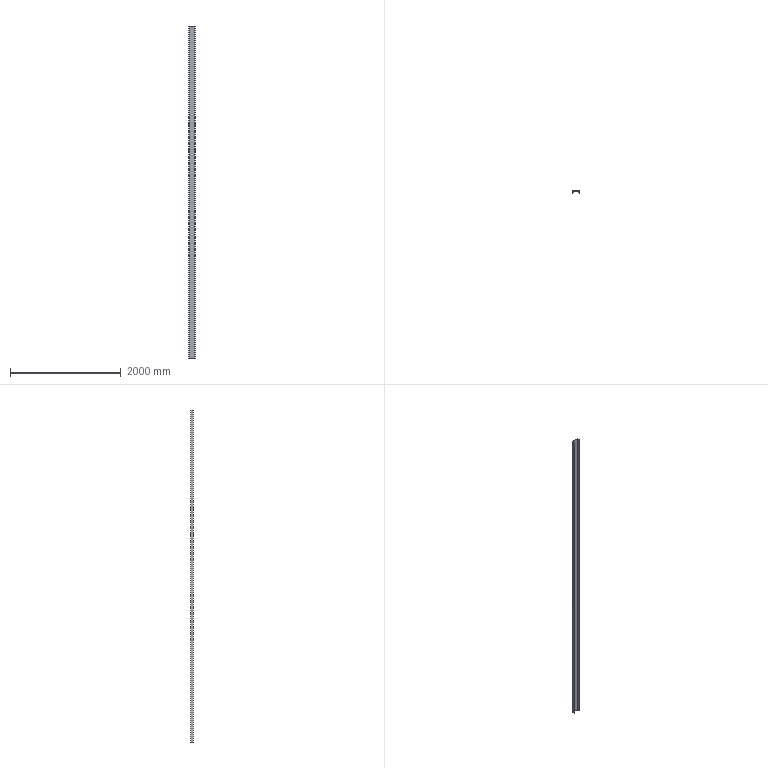Part | SolidWorks | features Extrusion 1 | 1 solid | 14 faces | box 120 x 50 x 6000 mm | volume 8487812 mm3 | plane 10 | cylinder 4 | commonest cylinder face diameters 4 x2 10 x2
STEP:
#1=CARTESIAN_POINT('',(0.,0.,0.));
#2=VERTEX_POINT('',#1);
#3=CARTESIAN_POINT('',(2.549,0.,0.));
#4=VERTEX_POINT('',#3);
#5=CARTESIAN_POINT('',(0.,0.,0.));
#6=DIRECTION('',(1.,0.,0.));
#7=VECTOR('',#6,1000.);
#8=LINE('',#5,#7);
#9=EDGE_CURVE('',#2,#4,#8,.T.);
#10=ORIENTED_EDGE('',*,*,#9,.T.);
#11=CARTESIAN_POINT('',(2.549,0.,6000.));
#12=VERTEX_POINT('',#11);
#13=CARTESIAN_POINT('',(2.549,0.,6000.));
#14=DIRECTION('',(0.,0.,-1.));
#15=VECTOR('',#14,1000.);
#16=LINE('',#13,#15);
#17=EDGE_CURVE('',#12,#4,#16,.T.);
#18=ORIENTED_EDGE('',*,*,#17,.F.);
#19=CARTESIAN_POINT('',(0.,0.,6000.));
#20=VERTEX_POINT('',#19);
#21=CARTESIAN_POINT('',(0.,0.,6000.));
#22=DIRECTION('',(1.,0.,0.));
#23=VECTOR('',#22,1000.);
#24=LINE('',#21,#23);
#25=EDGE_CURVE('',#20,#12,#24,.T.);
#26=ORIENTED_EDGE('',*,*,#25,.F.);
#27=CARTESIAN_POINT('',(0.,0.,6000.));
#28=DIRECTION('',(0.,0.,-1.));
#29=VECTOR('',#28,1000.);
#30=LINE('',#27,#29);
#31=EDGE_CURVE('',#20,#2,#30,.T.);
#32=ORIENTED_EDGE('',*,*,#31,.T.);
#33=EDGE_LOOP('',(#10,#18,#26,#32));
#34=FACE_OUTER_BOUND('',#33,.T.);
#35=CARTESIAN_POINT('',(0.,0.,6000.));
#36=DIRECTION('',(0.,1.,0.));
#37=DIRECTION('',(0.,0.,1.));
#38=AXIS2_PLACEMENT_3D('',#35,#36,#37);
#39=PLANE('',#38);
#40=ADVANCED_FACE('',(#34),#39,.F.);
#41=CARTESIAN_POINT('',(4.536,1.773,0.));
#42=VERTEX_POINT('',#41);
#43=CARTESIAN_POINT('',(2.549,2.,0.));
#44=DIRECTION('',(0.,0.,1.));
#45=DIRECTION('',(-1.,0.,0.));
#46=AXIS2_PLACEMENT_3D('',#43,#44,#45);
#47=CIRCLE('',#46,2.);
#48=EDGE_CURVE('',#4,#42,#47,.T.);
#49=ORIENTED_EDGE('',*,*,#48,.T.);
#50=CARTESIAN_POINT('',(4.536,1.773,6000.));
#51=VERTEX_POINT('',#50);
#52=CARTESIAN_POINT('',(4.536,1.773,6000.));
#53=DIRECTION('',(0.,0.,-1.));
#54=VECTOR('',#53,1000.);
#55=LINE('',#52,#54);
#56=EDGE_CURVE('',#51,#42,#55,.T.);
#57=ORIENTED_EDGE('',*,*,#56,.F.);
#58=CARTESIAN_POINT('',(2.549,2.,6000.));
#59=DIRECTION('',(0.,0.,1.));
#60=DIRECTION('',(-1.,0.,0.));
#61=AXIS2_PLACEMENT_3D('',#58,#59,#60);
#62=CIRCLE('',#61,2.);
#63=EDGE_CURVE('',#12,#51,#62,.T.);
#64=ORIENTED_EDGE('',*,*,#63,.F.);
#65=ORIENTED_EDGE('',*,*,#17,.T.);
#66=EDGE_LOOP('',(#49,#57,#64,#65));
#67=FACE_OUTER_BOUND('',#66,.T.);
#68=CARTESIAN_POINT('',(2.549,2.,6000.));
#69=DIRECTION('',(0.,0.,-1.));
#70=DIRECTION('',(-1.,0.,0.));
#71=AXIS2_PLACEMENT_3D('',#68,#69,#70);
#72=CYLINDRICAL_SURFACE('',#71,2.);
#73=ADVANCED_FACE('',(#67),#72,.T.);
#74=CARTESIAN_POINT('',(8.753,38.724,0.));
#75=VERTEX_POINT('',#74);
#76=CARTESIAN_POINT('',(4.536,1.773,0.));
#77=DIRECTION('',(0.1134,0.9936,0.));
#78=VECTOR('',#77,1000.);
#79=LINE('',#76,#78);
#80=EDGE_CURVE('',#42,#75,#79,.T.);
#81=ORIENTED_EDGE('',*,*,#80,.T.);
#82=CARTESIAN_POINT('',(8.753,38.724,6000.));
#83=VERTEX_POINT('',#82);
#84=CARTESIAN_POINT('',(8.753,38.724,6000.));
#85=DIRECTION('',(0.,0.,-1.));
#86=VECTOR('',#85,1000.);
#87=LINE('',#84,#86);
#88=EDGE_CURVE('',#83,#75,#87,.T.);
#89=ORIENTED_EDGE('',*,*,#88,.F.);
#90=CARTESIAN_POINT('',(4.536,1.773,6000.));
#91=DIRECTION('',(0.1134,0.9936,0.));
#92=VECTOR('',#91,1000.);
#93=LINE('',#90,#92);
#94=EDGE_CURVE('',#51,#83,#93,.T.);
#95=ORIENTED_EDGE('',*,*,#94,.F.);
#96=ORIENTED_EDGE('',*,*,#56,.T.);
#97=EDGE_LOOP('',(#81,#89,#95,#96));
#98=FACE_OUTER_BOUND('',#97,.T.);
#99=CARTESIAN_POINT('',(4.536,1.773,6000.));
#100=DIRECTION('',(-0.9936,0.1134,0.));
#101=DIRECTION('',(-0.1134,-0.9936,0.));
#102=AXIS2_PLACEMENT_3D('',#99,#100,#101);
#103=PLANE('',#102);
#104=ADVANCED_FACE('',(#98),#103,.F.);
#105=CARTESIAN_POINT('',(13.72,43.157,0.));
#106=VERTEX_POINT('',#105);
#107=CARTESIAN_POINT('',(13.72,38.157,0.));
#108=DIRECTION('',(0.,0.,-1.));
#109=DIRECTION('',(-1.,0.,0.));
#110=AXIS2_PLACEMENT_3D('',#107,#108,#109);
#111=CIRCLE('',#110,5.);
#112=EDGE_CURVE('',#75,#106,#111,.T.);
#113=ORIENTED_EDGE('',*,*,#112,.T.);
#114=CARTESIAN_POINT('',(13.72,43.157,6000.));
#115=VERTEX_POINT('',#114);
#116=CARTESIAN_POINT('',(13.72,43.157,6000.));
#117=DIRECTION('',(0.,0.,-1.));
#118=VECTOR('',#117,1000.);
#119=LINE('',#116,#118);
#120=EDGE_CURVE('',#115,#106,#119,.T.);
#121=ORIENTED_EDGE('',*,*,#120,.F.);
#122=CARTESIAN_POINT('',(13.72,38.157,6000.));
#123=DIRECTION('',(0.,0.,-1.));
#124=DIRECTION('',(-1.,0.,0.));
#125=AXIS2_PLACEMENT_3D('',#122,#123,#124);
#126=CIRCLE('',#125,5.);
#127=EDGE_CURVE('',#83,#115,#126,.T.);
#128=ORIENTED_EDGE('',*,*,#127,.F.);
#129=ORIENTED_EDGE('',*,*,#88,.T.);
#130=EDGE_LOOP('',(#113,#121,#128,#129));
#131=FACE_OUTER_BOUND('',#130,.T.);
#132=CARTESIAN_POINT('',(13.72,38.157,6000.));
#133=DIRECTION('',(0.,0.,-1.));
#134=DIRECTION('',(-1.,0.,0.));
#135=AXIS2_PLACEMENT_3D('',#132,#133,#134);
#136=CYLINDRICAL_SURFACE('',#135,5.);
#137=ADVANCED_FACE('',(#131),#136,.F.);
#138=CARTESIAN_POINT('',(106.28,43.157,0.));
#139=VERTEX_POINT('',#138);
#140=CARTESIAN_POINT('',(13.72,43.157,0.));
#141=DIRECTION('',(1.,0.,0.));
#142=VECTOR('',#141,1000.);
#143=LINE('',#140,#142);
#144=EDGE_CURVE('',#106,#139,#143,.T.);
#145=ORIENTED_EDGE('',*,*,#144,.T.);
#146=CARTESIAN_POINT('',(106.28,43.157,6000.));
#147=VERTEX_POINT('',#146);
#148=CARTESIAN_POINT('',(106.28,43.157,6000.));
#149=DIRECTION('',(0.,0.,-1.));
#150=VECTOR('',#149,1000.);
#151=LINE('',#148,#150);
#152=EDGE_CURVE('',#147,#139,#151,.T.);
#153=ORIENTED_EDGE('',*,*,#152,.F.);
#154=CARTESIAN_POINT('',(13.72,43.157,6000.));
#155=DIRECTION('',(1.,0.,0.));
#156=VECTOR('',#155,1000.);
#157=LINE('',#154,#156);
#158=EDGE_CURVE('',#115,#147,#157,.T.);
#159=ORIENTED_EDGE('',*,*,#158,.F.);
#160=ORIENTED_EDGE('',*,*,#120,.T.);
#161=EDGE_LOOP('',(#145,#153,#159,#160));
#162=FACE_OUTER_BOUND('',#161,.T.);
#163=CARTESIAN_POINT('',(13.72,43.157,6000.));
#164=DIRECTION('',(0.,1.,0.));
#165=DIRECTION('',(0.,0.,1.));
#166=AXIS2_PLACEMENT_3D('',#163,#164,#165);
#167=PLANE('',#166);
#168=ADVANCED_FACE('',(#162),#167,.F.);
#169=CARTESIAN_POINT('',(111.247,38.724,0.));
#170=VERTEX_POINT('',#169);
#171=CARTESIAN_POINT('',(106.28,38.157,0.));
#172=DIRECTION('',(0.,0.,-1.));
#173=DIRECTION('',(1.,0.,0.));
#174=AXIS2_PLACEMENT_3D('',#171,#172,#173);
#175=CIRCLE('',#174,5.);
#176=EDGE_CURVE('',#139,#170,#175,.T.);
#177=ORIENTED_EDGE('',*,*,#176,.T.);
#178=CARTESIAN_POINT('',(111.247,38.724,6000.));
#179=VERTEX_POINT('',#178);
#180=CARTESIAN_POINT('',(111.247,38.724,6000.));
#181=DIRECTION('',(0.,0.,-1.));
#182=VECTOR('',#181,1000.);
#183=LINE('',#180,#182);
#184=EDGE_CURVE('',#179,#170,#183,.T.);
#185=ORIENTED_EDGE('',*,*,#184,.F.);
#186=CARTESIAN_POINT('',(106.28,38.157,6000.));
#187=DIRECTION('',(0.,0.,-1.));
#188=DIRECTION('',(1.,0.,0.));
#189=AXIS2_PLACEMENT_3D('',#186,#187,#188);
#190=CIRCLE('',#189,5.);
#191=EDGE_CURVE('',#147,#179,#190,.T.);
#192=ORIENTED_EDGE('',*,*,#191,.F.);
#193=ORIENTED_EDGE('',*,*,#152,.T.);
#194=EDGE_LOOP('',(#177,#185,#192,#193));
#195=FACE_OUTER_BOUND('',#194,.T.);
#196=CARTESIAN_POINT('',(106.28,38.157,6000.));
#197=DIRECTION('',(0.,0.,-1.));
#198=DIRECTION('',(-1.,0.,0.));
#199=AXIS2_PLACEMENT_3D('',#196,#197,#198);
#200=CYLINDRICAL_SURFACE('',#199,5.);
#201=ADVANCED_FACE('',(#195),#200,.F.);
#202=CARTESIAN_POINT('',(115.464,1.773,0.));
#203=VERTEX_POINT('',#202);
#204=CARTESIAN_POINT('',(115.464,1.773,0.));
#205=DIRECTION('',(0.1134,-0.9936,0.));
#206=VECTOR('',#205,1000.);
#207=LINE('',#204,#206);
#208=EDGE_CURVE('',#170,#203,#207,.T.);
#209=ORIENTED_EDGE('',*,*,#208,.T.);
#210=CARTESIAN_POINT('',(115.464,1.773,6000.));
#211=VERTEX_POINT('',#210);
#212=CARTESIAN_POINT('',(115.464,1.773,6000.));
#213=DIRECTION('',(0.,0.,-1.));
#214=VECTOR('',#213,1000.);
#215=LINE('',#212,#214);
#216=EDGE_CURVE('',#211,#203,#215,.T.);
#217=ORIENTED_EDGE('',*,*,#216,.F.);
#218=CARTESIAN_POINT('',(115.464,1.773,6000.));
#219=DIRECTION('',(0.1134,-0.9936,0.));
#220=VECTOR('',#219,1000.);
#221=LINE('',#218,#220);
#222=EDGE_CURVE('',#179,#211,#221,.T.);
#223=ORIENTED_EDGE('',*,*,#222,.F.);
#224=ORIENTED_EDGE('',*,*,#184,.T.);
#225=EDGE_LOOP('',(#209,#217,#223,#224));
#226=FACE_OUTER_BOUND('',#225,.T.);
#227=CARTESIAN_POINT('',(115.464,1.773,6000.));
#228=DIRECTION('',(0.9936,0.1134,0.));
#229=DIRECTION('',(-0.1134,0.9936,0.));
#230=AXIS2_PLACEMENT_3D('',#227,#228,#229);
#231=PLANE('',#230);
#232=ADVANCED_FACE('',(#226),#231,.F.);
#233=CARTESIAN_POINT('',(117.451,0.,0.));
#234=VERTEX_POINT('',#233);
#235=CARTESIAN_POINT('',(117.451,2.,0.));
#236=DIRECTION('',(0.,0.,1.));
#237=DIRECTION('',(1.,0.,0.));
#238=AXIS2_PLACEMENT_3D('',#235,#236,#237);
#239=CIRCLE('',#238,2.);
#240=EDGE_CURVE('',#203,#234,#239,.T.);
#241=ORIENTED_EDGE('',*,*,#240,.T.);
#242=CARTESIAN_POINT('',(117.451,0.,6000.));
#243=VERTEX_POINT('',#242);
#244=CARTESIAN_POINT('',(117.451,0.,6000.));
#245=DIRECTION('',(0.,0.,-1.));
#246=VECTOR('',#245,1000.);
#247=LINE('',#244,#246);
#248=EDGE_CURVE('',#243,#234,#247,.T.);
#249=ORIENTED_EDGE('',*,*,#248,.F.);
#250=CARTESIAN_POINT('',(117.451,2.,6000.));
#251=DIRECTION('',(0.,0.,1.));
#252=DIRECTION('',(1.,0.,0.));
#253=AXIS2_PLACEMENT_3D('',#250,#251,#252);
#254=CIRCLE('',#253,2.);
#255=EDGE_CURVE('',#211,#243,#254,.T.);
#256=ORIENTED_EDGE('',*,*,#255,.F.);
#257=ORIENTED_EDGE('',*,*,#216,.T.);
#258=EDGE_LOOP('',(#241,#249,#256,#257));
#259=FACE_OUTER_BOUND('',#258,.T.);
#260=CARTESIAN_POINT('',(117.451,2.,6000.));
#261=DIRECTION('',(0.,0.,-1.));
#262=DIRECTION('',(-1.,0.,0.));
#263=AXIS2_PLACEMENT_3D('',#260,#261,#262);
#264=CYLINDRICAL_SURFACE('',#263,2.);
#265=ADVANCED_FACE('',(#259),#264,.T.);
#266=CARTESIAN_POINT('',(120.,0.,0.));
#267=VERTEX_POINT('',#266);
#268=CARTESIAN_POINT('',(120.,0.,0.));
#269=DIRECTION('',(1.,0.,0.));
#270=VECTOR('',#269,1000.);
#271=LINE('',#268,#270);
#272=EDGE_CURVE('',#234,#267,#271,.T.);
#273=ORIENTED_EDGE('',*,*,#272,.T.);
#274=CARTESIAN_POINT('',(120.,0.,6000.));
#275=VERTEX_POINT('',#274);
#276=CARTESIAN_POINT('',(120.,0.,6000.));
#277=DIRECTION('',(0.,0.,-1.));
#278=VECTOR('',#277,1000.);
#279=LINE('',#276,#278);
#280=EDGE_CURVE('',#275,#267,#279,.T.);
#281=ORIENTED_EDGE('',*,*,#280,.F.);
#282=CARTESIAN_POINT('',(120.,0.,6000.));
#283=DIRECTION('',(1.,0.,0.));
#284=VECTOR('',#283,1000.);
#285=LINE('',#282,#284);
#286=EDGE_CURVE('',#243,#275,#285,.T.);
#287=ORIENTED_EDGE('',*,*,#286,.F.);
#288=ORIENTED_EDGE('',*,*,#248,.T.);
#289=EDGE_LOOP('',(#273,#281,#287,#288));
#290=FACE_OUTER_BOUND('',#289,.T.);
#291=CARTESIAN_POINT('',(120.,0.,6000.));
#292=DIRECTION('',(0.,1.,0.));
#293=DIRECTION('',(0.,0.,1.));
#294=AXIS2_PLACEMENT_3D('',#291,#292,#293);
#295=PLANE('',#294);
#296=ADVANCED_FACE('',(#290),#295,.F.);
#297=CARTESIAN_POINT('',(120.,50.,0.));
#298=VERTEX_POINT('',#297);
#299=CARTESIAN_POINT('',(120.,50.,0.));
#300=DIRECTION('',(0.,1.,0.));
#301=VECTOR('',#300,1000.);
#302=LINE('',#299,#301);
#303=EDGE_CURVE('',#267,#298,#302,.T.);
#304=ORIENTED_EDGE('',*,*,#303,.T.);
#305=CARTESIAN_POINT('',(120.,50.,6000.));
#306=VERTEX_POINT('',#305);
#307=CARTESIAN_POINT('',(120.,50.,6000.));
#308=DIRECTION('',(0.,0.,-1.));
#309=VECTOR('',#308,1000.);
#310=LINE('',#307,#309);
#311=EDGE_CURVE('',#306,#298,#310,.T.);
#312=ORIENTED_EDGE('',*,*,#311,.F.);
#313=CARTESIAN_POINT('',(120.,50.,6000.));
#314=DIRECTION('',(0.,1.,0.));
#315=VECTOR('',#314,1000.);
#316=LINE('',#313,#315);
#317=EDGE_CURVE('',#275,#306,#316,.T.);
#318=ORIENTED_EDGE('',*,*,#317,.F.);
#319=ORIENTED_EDGE('',*,*,#280,.T.);
#320=EDGE_LOOP('',(#304,#312,#318,#319));
#321=FACE_OUTER_BOUND('',#320,.T.);
#322=CARTESIAN_POINT('',(120.,50.,6000.));
#323=DIRECTION('',(-1.,0.,0.));
#324=DIRECTION('',(0.,-1.,0.));
#325=AXIS2_PLACEMENT_3D('',#322,#323,#324);
#326=PLANE('',#325);
#327=ADVANCED_FACE('',(#321),#326,.F.);
#328=CARTESIAN_POINT('',(0.,50.,0.));
#329=VERTEX_POINT('',#328);
#330=CARTESIAN_POINT('',(0.,50.,0.));
#331=DIRECTION('',(-1.,0.,0.));
#332=VECTOR('',#331,1000.);
#333=LINE('',#330,#332);
#334=EDGE_CURVE('',#298,#329,#333,.T.);
#335=ORIENTED_EDGE('',*,*,#334,.T.);
#336=CARTESIAN_POINT('',(0.,50.,6000.));
#337=VERTEX_POINT('',#336);
#338=CARTESIAN_POINT('',(0.,50.,6000.));
#339=DIRECTION('',(0.,0.,-1.));
#340=VECTOR('',#339,1000.);
#341=LINE('',#338,#340);
#342=EDGE_CURVE('',#337,#329,#341,.T.);
#343=ORIENTED_EDGE('',*,*,#342,.F.);
#344=CARTESIAN_POINT('',(0.,50.,6000.));
#345=DIRECTION('',(-1.,0.,0.));
#346=VECTOR('',#345,1000.);
#347=LINE('',#344,#346);
#348=EDGE_CURVE('',#306,#337,#347,.T.);
#349=ORIENTED_EDGE('',*,*,#348,.F.);
#350=ORIENTED_EDGE('',*,*,#311,.T.);
#351=EDGE_LOOP('',(#335,#343,#349,#350));
#352=FACE_OUTER_BOUND('',#351,.T.);
#353=CARTESIAN_POINT('',(0.,50.,6000.));
#354=DIRECTION('',(0.,-1.,0.));
#355=DIRECTION('',(0.,0.,-1.));
#356=AXIS2_PLACEMENT_3D('',#353,#354,#355);
#357=PLANE('',#356);
#358=ADVANCED_FACE('',(#352),#357,.F.);
#359=CARTESIAN_POINT('',(0.,0.,0.));
#360=DIRECTION('',(0.,-1.,0.));
#361=VECTOR('',#360,1000.);
#362=LINE('',#359,#361);
#363=EDGE_CURVE('',#329,#2,#362,.T.);
#364=ORIENTED_EDGE('',*,*,#363,.T.);
#365=ORIENTED_EDGE('',*,*,#31,.F.);
#366=CARTESIAN_POINT('',(0.,0.,6000.));
#367=DIRECTION('',(0.,-1.,0.));
#368=VECTOR('',#367,1000.);
#369=LINE('',#366,#368);
#370=EDGE_CURVE('',#337,#20,#369,.T.);
#371=ORIENTED_EDGE('',*,*,#370,.F.);
#372=ORIENTED_EDGE('',*,*,#342,.T.);
#373=EDGE_LOOP('',(#364,#365,#371,#372));
#374=FACE_OUTER_BOUND('',#373,.T.);
#375=CARTESIAN_POINT('',(0.,0.,6000.));
#376=DIRECTION('',(1.,0.,0.));
#377=DIRECTION('',(0.,0.,-1.));
#378=AXIS2_PLACEMENT_3D('',#375,#376,#377);
#379=PLANE('',#378);
#380=ADVANCED_FACE('',(#374),#379,.F.);
#381=ORIENTED_EDGE('',*,*,#25,.T.);
#382=ORIENTED_EDGE('',*,*,#63,.T.);
#383=ORIENTED_EDGE('',*,*,#94,.T.);
#384=ORIENTED_EDGE('',*,*,#127,.T.);
#385=ORIENTED_EDGE('',*,*,#158,.T.);
#386=ORIENTED_EDGE('',*,*,#191,.T.);
#387=ORIENTED_EDGE('',*,*,#222,.T.);
#388=ORIENTED_EDGE('',*,*,#255,.T.);
#389=ORIENTED_EDGE('',*,*,#286,.T.);
#390=ORIENTED_EDGE('',*,*,#317,.T.);
#391=ORIENTED_EDGE('',*,*,#348,.T.);
#392=ORIENTED_EDGE('',*,*,#370,.T.);
#393=EDGE_LOOP('',(#381,#382,#383,#384,#385,#386,#387,#388,#389,#390,#391,#392));
#394=FACE_OUTER_BOUND('',#393,.T.);
#395=CARTESIAN_POINT('',(2.549,2.,6000.));
#396=DIRECTION('',(0.,0.,-1.));
#397=DIRECTION('',(-1.,0.,0.));
#398=AXIS2_PLACEMENT_3D('',#395,#396,#397);
#399=PLANE('',#398);
#400=ADVANCED_FACE('',(#394),#399,.F.);
#401=ORIENTED_EDGE('',*,*,#9,.F.);
#402=ORIENTED_EDGE('',*,*,#363,.F.);
#403=ORIENTED_EDGE('',*,*,#334,.F.);
#404=ORIENTED_EDGE('',*,*,#303,.F.);
#405=ORIENTED_EDGE('',*,*,#272,.F.);
#406=ORIENTED_EDGE('',*,*,#240,.F.);
#407=ORIENTED_EDGE('',*,*,#208,.F.);
#408=ORIENTED_EDGE('',*,*,#176,.F.);
#409=ORIENTED_EDGE('',*,*,#144,.F.);
#410=ORIENTED_EDGE('',*,*,#112,.F.);
#411=ORIENTED_EDGE('',*,*,#80,.F.);
#412=ORIENTED_EDGE('',*,*,#48,.F.);
#413=EDGE_LOOP('',(#401,#402,#403,#404,#405,#406,#407,#408,#409,#410,#411,#412));
#414=FACE_OUTER_BOUND('',#413,.T.);
#415=CARTESIAN_POINT('',(2.549,2.,0.));
#416=DIRECTION('',(0.,0.,-1.));
#417=DIRECTION('',(-1.,0.,0.));
#418=AXIS2_PLACEMENT_3D('',#415,#416,#417);
#419=PLANE('',#418);
#420=ADVANCED_FACE('',(#414),#419,.T.);
#421=CLOSED_SHELL('',(#40,#73,#104,#137,#168,#201,#232,#265,#296,#327,#358,#380,#400,#420));
#422=MANIFOLD_SOLID_BREP('',#421);
#423=CARTESIAN_POINT('',(0.,0.,0.));
#424=DIRECTION('',(0.,0.,1.));
#425=DIRECTION('',(1.,0.,0.));
#426=AXIS2_PLACEMENT_3D('',#423,#424,#425);
#427=(LENGTH_UNIT()NAMED_UNIT(*)SI_UNIT(.MILLI.,.METRE.));
#428=UNCERTAINTY_MEASURE_WITH_UNIT(LENGTH_MEASURE(0.00001),#427,'','');
#429=(NAMED_UNIT(*)PLANE_ANGLE_UNIT()SI_UNIT($,.RADIAN.));
#430=(NAMED_UNIT(*)SI_UNIT($,.STERADIAN.)SOLID_ANGLE_UNIT());
#431=(GEOMETRIC_REPRESENTATION_CONTEXT(3)GLOBAL_UNCERTAINTY_ASSIGNED_CONTEXT((#428))GLOBAL_UNIT_ASSIGNED_CONTEXT((#427,#429,#430))REPRESENTATION_CONTEXT('',''));
#432=ADVANCED_BREP_SHAPE_REPRESENTATION('',(#422,#426),#431);